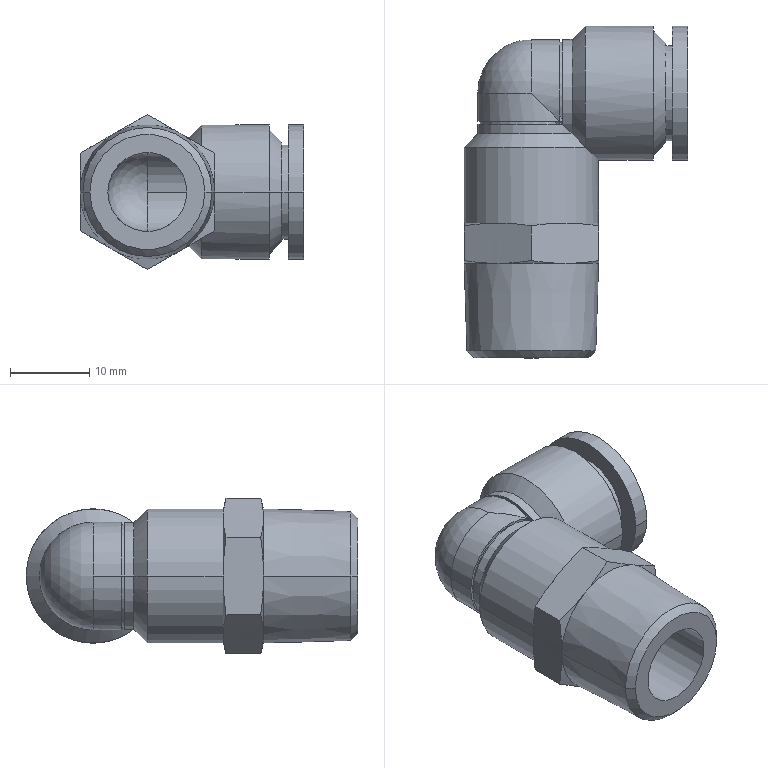Part | NX | 1 solid | 74 faces | box 28.304 x 42 x 19.63 mm | volume 6609 mm3 | cylinder 32 | cone 21 | plane 19 | sphere 2 | commonest cylinder face diameters 13.6 x12 12.92 x8 17 x6 10 x4 12 x2